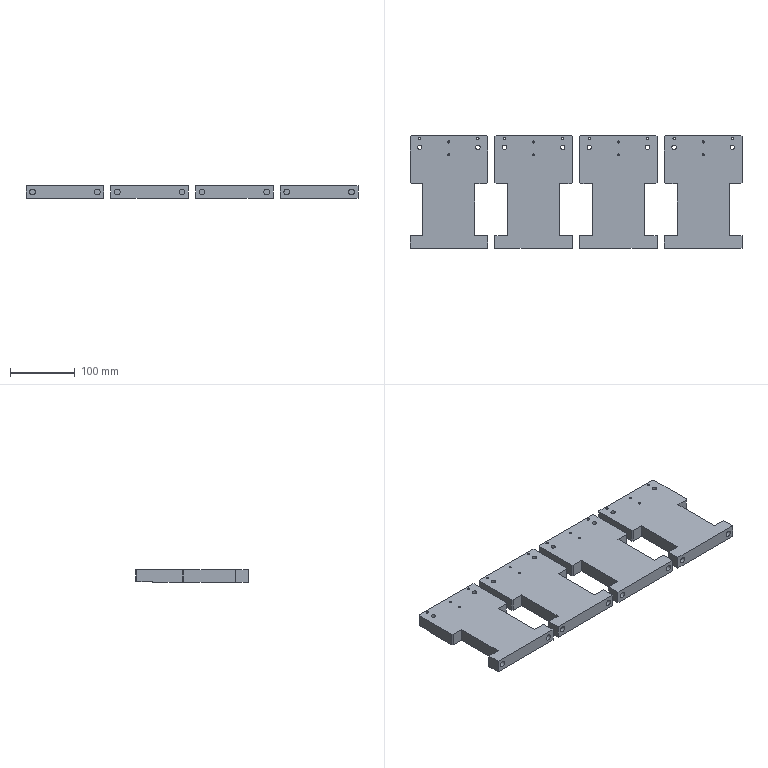Part | 4 solids | 112 faces | box 513 x 174.5 x 20 mm | volume 1381058 mm3 | plane 80 | cylinder 32 | commonest cylinder face diameters 3.3 x8 3.6 x8 7 x8 9 x8